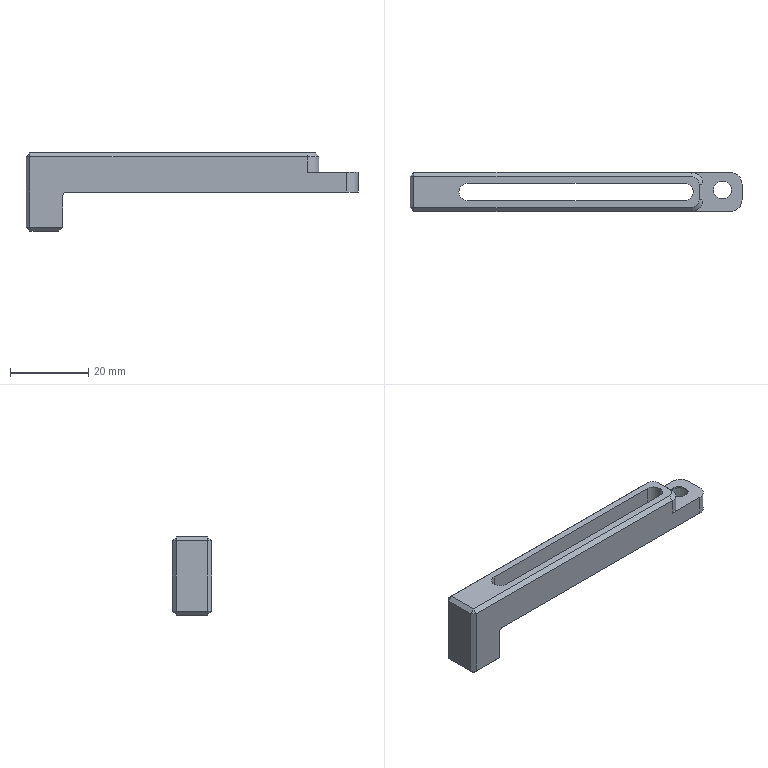Part | SolidWorks | features ICE 4, Fillet 2, HoleWzd 2, Chamfer 1, Extrusion 1 | 1 solid | 51 faces | box 85 x 10 x 20 mm | volume 4776 mm3 | plane 30 | cylinder 17 | cone 4 | commonest cylinder face diameters 4.5 x5 8 x5 6 x4 5 x2 2 x1
STEP:
#1=CARTESIAN_POINT('',(41.5,5.5,-0.4));
#2=VERTEX_POINT('',#1);
#3=CARTESIAN_POINT('',(33.5,5.5,-0.4));
#4=VERTEX_POINT('',#3);
#5=CARTESIAN_POINT('',(37.5,5.5,-0.4));
#6=DIRECTION('',(0.,0.,-1.));
#7=DIRECTION('',(-1.,0.,0.));
#8=AXIS2_PLACEMENT_3D('',#5,#6,#7);
#9=CIRCLE('',#8,4.);
#10=EDGE_CURVE('',#2,#4,#9,.T.);
#11=ORIENTED_EDGE('',*,*,#10,.F.);
#12=CARTESIAN_POINT('',(41.5,5.5,-5.));
#13=VERTEX_POINT('',#12);
#14=CARTESIAN_POINT('',(41.5,5.5,-5.));
#15=DIRECTION('',(0.,0.,-1.));
#16=VECTOR('',#15,1000.);
#17=LINE('',#14,#16);
#18=EDGE_CURVE('',#2,#13,#17,.T.);
#19=ORIENTED_EDGE('',*,*,#18,.T.);
#20=CARTESIAN_POINT('',(33.5,5.5,-5.));
#21=VERTEX_POINT('',#20);
#22=CARTESIAN_POINT('',(37.5,5.5,-5.));
#23=DIRECTION('',(0.,0.,-1.));
#24=DIRECTION('',(-1.,0.,0.));
#25=AXIS2_PLACEMENT_3D('',#22,#23,#24);
#26=CIRCLE('',#25,4.);
#27=EDGE_CURVE('',#13,#21,#26,.T.);
#28=ORIENTED_EDGE('',*,*,#27,.T.);
#29=CARTESIAN_POINT('',(33.5,5.5,-5.));
#30=DIRECTION('',(0.,0.,-1.));
#31=VECTOR('',#30,1000.);
#32=LINE('',#29,#31);
#33=EDGE_CURVE('',#4,#21,#32,.T.);
#34=ORIENTED_EDGE('',*,*,#33,.F.);
#35=EDGE_LOOP('',(#11,#19,#28,#34));
#36=FACE_OUTER_BOUND('',#35,.T.);
#37=CARTESIAN_POINT('',(37.5,5.5,-5.));
#38=DIRECTION('',(0.,0.,-1.));
#39=DIRECTION('',(-1.,0.,0.));
#40=AXIS2_PLACEMENT_3D('',#37,#38,#39);
#41=CYLINDRICAL_SURFACE('',#40,4.);
#42=ADVANCED_FACE('',(#36),#41,.F.);
#43=CARTESIAN_POINT('',(39.75,5.5,0.));
#44=VERTEX_POINT('',#43);
#45=CARTESIAN_POINT('',(35.25,5.5,0.));
#46=VERTEX_POINT('',#45);
#47=CARTESIAN_POINT('',(37.5,5.5,0.));
#48=DIRECTION('',(0.,0.,-1.));
#49=DIRECTION('',(-1.,0.,0.));
#50=AXIS2_PLACEMENT_3D('',#47,#48,#49);
#51=CIRCLE('',#50,2.25);
#52=EDGE_CURVE('',#44,#46,#51,.T.);
#53=ORIENTED_EDGE('',*,*,#52,.F.);
#54=CARTESIAN_POINT('',(39.75,5.5,-0.4));
#55=VERTEX_POINT('',#54);
#56=CARTESIAN_POINT('',(39.75,5.5,-5.));
#57=DIRECTION('',(0.,0.,-1.));
#58=VECTOR('',#57,1000.);
#59=LINE('',#56,#58);
#60=EDGE_CURVE('',#44,#55,#59,.T.);
#61=ORIENTED_EDGE('',*,*,#60,.T.);
#62=CARTESIAN_POINT('',(35.25,5.5,-0.4));
#63=VERTEX_POINT('',#62);
#64=CARTESIAN_POINT('',(37.5,5.5,-0.4));
#65=DIRECTION('',(0.,0.,-1.));
#66=DIRECTION('',(-1.,0.,0.));
#67=AXIS2_PLACEMENT_3D('',#64,#65,#66);
#68=CIRCLE('',#67,2.25);
#69=EDGE_CURVE('',#55,#63,#68,.T.);
#70=ORIENTED_EDGE('',*,*,#69,.T.);
#71=CARTESIAN_POINT('',(35.25,5.5,-5.));
#72=DIRECTION('',(0.,0.,-1.));
#73=VECTOR('',#72,1000.);
#74=LINE('',#71,#73);
#75=EDGE_CURVE('',#46,#63,#74,.T.);
#76=ORIENTED_EDGE('',*,*,#75,.F.);
#77=EDGE_LOOP('',(#53,#61,#70,#76));
#78=FACE_OUTER_BOUND('',#77,.T.);
#79=CARTESIAN_POINT('',(37.5,5.5,-5.));
#80=DIRECTION('',(0.,0.,-1.));
#81=DIRECTION('',(-1.,0.,0.));
#82=AXIS2_PLACEMENT_3D('',#79,#80,#81);
#83=CYLINDRICAL_SURFACE('',#82,2.25);
#84=ADVANCED_FACE('',(#78),#83,.F.);
#85=CARTESIAN_POINT('',(-35.3,4.802,-10.));
#86=VERTEX_POINT('',#85);
#87=CARTESIAN_POINT('',(-40.3,4.802,-10.));
#88=VERTEX_POINT('',#87);
#89=CARTESIAN_POINT('',(-37.8,4.802,-10.));
#90=DIRECTION('',(0.,0.,-1.));
#91=DIRECTION('',(-1.,0.,0.));
#92=AXIS2_PLACEMENT_3D('',#89,#90,#91);
#93=CIRCLE('',#92,2.5);
#94=EDGE_CURVE('',#86,#88,#93,.T.);
#95=ORIENTED_EDGE('',*,*,#94,.F.);
#96=CARTESIAN_POINT('',(-35.3,4.802,-15.));
#97=VERTEX_POINT('',#96);
#98=CARTESIAN_POINT('',(-35.3,4.802,-15.));
#99=DIRECTION('',(0.,0.,-1.));
#100=VECTOR('',#99,1000.);
#101=LINE('',#98,#100);
#102=EDGE_CURVE('',#86,#97,#101,.T.);
#103=ORIENTED_EDGE('',*,*,#102,.T.);
#104=CARTESIAN_POINT('',(-40.3,4.802,-15.));
#105=VERTEX_POINT('',#104);
#106=CARTESIAN_POINT('',(-37.8,4.802,-15.));
#107=DIRECTION('',(0.,0.,-1.));
#108=DIRECTION('',(-1.,0.,0.));
#109=AXIS2_PLACEMENT_3D('',#106,#107,#108);
#110=CIRCLE('',#109,2.5);
#111=EDGE_CURVE('',#97,#105,#110,.T.);
#112=ORIENTED_EDGE('',*,*,#111,.T.);
#113=CARTESIAN_POINT('',(-40.3,4.802,-15.));
#114=DIRECTION('',(0.,0.,-1.));
#115=VECTOR('',#114,1000.);
#116=LINE('',#113,#115);
#117=EDGE_CURVE('',#88,#105,#116,.T.);
#118=ORIENTED_EDGE('',*,*,#117,.F.);
#119=EDGE_LOOP('',(#95,#103,#112,#118));
#120=FACE_OUTER_BOUND('',#119,.T.);
#121=CARTESIAN_POINT('',(-37.8,4.802,-15.));
#122=DIRECTION('',(0.,0.,-1.));
#123=DIRECTION('',(-1.,0.,0.));
#124=AXIS2_PLACEMENT_3D('',#121,#122,#123);
#125=CYLINDRICAL_SURFACE('',#124,2.5);
#126=ADVANCED_FACE('',(#120),#125,.F.);
#127=CARTESIAN_POINT('',(-37.8,4.802,-8.498));
#128=VERTEX_POINT('',#127);
#129=CARTESIAN_POINT('',(-40.3,4.802,-10.));
#130=DIRECTION('',(-0.8572,0.,-0.515));
#131=VECTOR('',#130,1000.);
#132=LINE('',#129,#131);
#133=EDGE_CURVE('',#128,#88,#132,.T.);
#134=ORIENTED_EDGE('',*,*,#133,.F.);
#135=CARTESIAN_POINT('',(-35.3,4.802,-10.));
#136=DIRECTION('',(0.8572,0.,-0.515));
#137=VECTOR('',#136,1000.);
#138=LINE('',#135,#137);
#139=EDGE_CURVE('',#128,#86,#138,.T.);
#140=ORIENTED_EDGE('',*,*,#139,.T.);
#141=ORIENTED_EDGE('',*,*,#94,.T.);
#142=EDGE_LOOP('',(#134,#140,#141));
#143=FACE_OUTER_BOUND('',#142,.T.);
#144=CARTESIAN_POINT('',(-37.8,4.802,-10.));
#145=DIRECTION('',(0.,0.,-1.));
#146=DIRECTION('',(-1.,0.,0.));
#147=AXIS2_PLACEMENT_3D('',#144,#145,#146);
#148=CONICAL_SURFACE('',#147,2.5,1.03);
#149=ADVANCED_FACE('',(#143),#148,.F.);
#150=CARTESIAN_POINT('',(-30.,5.,5.));
#151=VERTEX_POINT('',#150);
#152=CARTESIAN_POINT('',(-27.75,7.25,5.));
#153=VERTEX_POINT('',#152);
#154=CARTESIAN_POINT('',(-27.75,5.,5.));
#155=DIRECTION('',(0.,0.,-1.));
#156=DIRECTION('',(-1.,0.,0.));
#157=AXIS2_PLACEMENT_3D('',#154,#155,#156);
#158=CIRCLE('',#157,2.25);
#159=EDGE_CURVE('',#151,#153,#158,.T.);
#160=ORIENTED_EDGE('',*,*,#159,.F.);
#161=CARTESIAN_POINT('',(-30.,5.,-0.6));
#162=VERTEX_POINT('',#161);
#163=CARTESIAN_POINT('',(-30.,5.,5.));
#164=DIRECTION('',(0.,0.,-1.));
#165=VECTOR('',#164,1000.);
#166=LINE('',#163,#165);
#167=EDGE_CURVE('',#151,#162,#166,.T.);
#168=ORIENTED_EDGE('',*,*,#167,.T.);
#169=CARTESIAN_POINT('',(-27.75,7.25,-0.6));
#170=VERTEX_POINT('',#169);
#171=CARTESIAN_POINT('',(-27.75,5.,-0.6));
#172=DIRECTION('',(0.,0.,-1.));
#173=DIRECTION('',(-1.,0.,0.));
#174=AXIS2_PLACEMENT_3D('',#171,#172,#173);
#175=CIRCLE('',#174,2.25);
#176=EDGE_CURVE('',#162,#170,#175,.T.);
#177=ORIENTED_EDGE('',*,*,#176,.T.);
#178=CARTESIAN_POINT('',(-27.75,7.25,5.));
#179=DIRECTION('',(0.,0.,-1.));
#180=VECTOR('',#179,1000.);
#181=LINE('',#178,#180);
#182=EDGE_CURVE('',#153,#170,#181,.T.);
#183=ORIENTED_EDGE('',*,*,#182,.F.);
#184=EDGE_LOOP('',(#160,#168,#177,#183));
#185=FACE_OUTER_BOUND('',#184,.T.);
#186=CARTESIAN_POINT('',(-27.75,5.,5.));
#187=DIRECTION('',(0.,0.,-1.));
#188=DIRECTION('',(-1.,0.,0.));
#189=AXIS2_PLACEMENT_3D('',#186,#187,#188);
#190=CYLINDRICAL_SURFACE('',#189,2.25);
#191=ADVANCED_FACE('',(#185),#190,.F.);
#192=CARTESIAN_POINT('',(-27.75,9.,-0.6));
#193=VERTEX_POINT('',#192);
#194=CARTESIAN_POINT('',(-31.75,5.,-0.6));
#195=VERTEX_POINT('',#194);
#196=CARTESIAN_POINT('',(-27.75,5.,-0.6));
#197=DIRECTION('',(0.,0.,1.));
#198=DIRECTION('',(1.,0.,0.));
#199=AXIS2_PLACEMENT_3D('',#196,#197,#198);
#200=CIRCLE('',#199,4.);
#201=EDGE_CURVE('',#193,#195,#200,.T.);
#202=ORIENTED_EDGE('',*,*,#201,.T.);
#203=CARTESIAN_POINT('',(-31.75,5.,-5.));
#204=VERTEX_POINT('',#203);
#205=CARTESIAN_POINT('',(-31.75,5.,-0.6));
#206=DIRECTION('',(0.,0.,-1.));
#207=VECTOR('',#206,1000.);
#208=LINE('',#205,#207);
#209=EDGE_CURVE('',#195,#204,#208,.T.);
#210=ORIENTED_EDGE('',*,*,#209,.T.);
#211=CARTESIAN_POINT('',(-27.75,9.,-5.));
#212=VERTEX_POINT('',#211);
#213=CARTESIAN_POINT('',(-27.75,5.,-5.));
#214=DIRECTION('',(0.,0.,1.));
#215=DIRECTION('',(1.,0.,0.));
#216=AXIS2_PLACEMENT_3D('',#213,#214,#215);
#217=CIRCLE('',#216,4.);
#218=EDGE_CURVE('',#212,#204,#217,.T.);
#219=ORIENTED_EDGE('',*,*,#218,.F.);
#220=CARTESIAN_POINT('',(-27.75,9.,-0.6));
#221=DIRECTION('',(0.,0.,-1.));
#222=VECTOR('',#221,1000.);
#223=LINE('',#220,#222);
#224=EDGE_CURVE('',#193,#212,#223,.T.);
#225=ORIENTED_EDGE('',*,*,#224,.F.);
#226=EDGE_LOOP('',(#202,#210,#219,#225));
#227=FACE_OUTER_BOUND('',#226,.T.);
#228=CARTESIAN_POINT('',(-27.75,5.,-0.6));
#229=DIRECTION('',(0.,0.,-1.));
#230=DIRECTION('',(-1.,0.,0.));
#231=AXIS2_PLACEMENT_3D('',#228,#229,#230);
#232=CYLINDRICAL_SURFACE('',#231,4.);
#233=ADVANCED_FACE('',(#227),#232,.F.);
#234=CARTESIAN_POINT('',(37.5,5.5,-5.));
#235=DIRECTION('',(0.,0.,-1.));
#236=DIRECTION('',(-1.,0.,0.));
#237=AXIS2_PLACEMENT_3D('',#234,#235,#236);
#238=CIRCLE('',#237,4.);
#239=EDGE_CURVE('',#21,#13,#238,.T.);
#240=ORIENTED_EDGE('',*,*,#239,.F.);
#241=ORIENTED_EDGE('',*,*,#27,.F.);
#242=EDGE_LOOP('',(#240,#241));
#243=FACE_BOUND('',#242,.T.);
#244=ORIENTED_EDGE('',*,*,#218,.T.);
#245=CARTESIAN_POINT('',(-27.75,1.,-5.));
#246=VERTEX_POINT('',#245);
#247=CARTESIAN_POINT('',(-27.75,5.,-5.));
#248=DIRECTION('',(0.,0.,1.));
#249=DIRECTION('',(1.,0.,0.));
#250=AXIS2_PLACEMENT_3D('',#247,#248,#249);
#251=CIRCLE('',#250,4.);
#252=EDGE_CURVE('',#204,#246,#251,.T.);
#253=ORIENTED_EDGE('',*,*,#252,.T.);
#254=CARTESIAN_POINT('',(27.75,1.,-5.));
#255=VERTEX_POINT('',#254);
#256=CARTESIAN_POINT('',(-27.75,1.,-5.));
#257=DIRECTION('',(1.,0.,0.));
#258=VECTOR('',#257,1000.);
#259=LINE('',#256,#258);
#260=EDGE_CURVE('',#246,#255,#259,.T.);
#261=ORIENTED_EDGE('',*,*,#260,.T.);
#262=CARTESIAN_POINT('',(27.75,9.,-5.));
#263=VERTEX_POINT('',#262);
#264=CARTESIAN_POINT('',(27.75,5.,-5.));
#265=DIRECTION('',(0.,0.,1.));
#266=DIRECTION('',(1.,0.,0.));
#267=AXIS2_PLACEMENT_3D('',#264,#265,#266);
#268=CIRCLE('',#267,4.);
#269=EDGE_CURVE('',#255,#263,#268,.T.);
#270=ORIENTED_EDGE('',*,*,#269,.T.);
#271=CARTESIAN_POINT('',(-27.75,9.,-5.));
#272=DIRECTION('',(-1.,0.,0.));
#273=VECTOR('',#272,1000.);
#274=LINE('',#271,#273);
#275=EDGE_CURVE('',#263,#212,#274,.T.);
#276=ORIENTED_EDGE('',*,*,#275,.T.);
#277=EDGE_LOOP('',(#244,#253,#261,#270,#276));
#278=FACE_BOUND('',#277,.T.);
#279=CARTESIAN_POINT('',(39.5,0.,-5.));
#280=VERTEX_POINT('',#279);
#281=CARTESIAN_POINT('',(-32.1,0.,-5.));
#282=VERTEX_POINT('',#281);
#283=CARTESIAN_POINT('',(42.5,0.,-5.));
#284=DIRECTION('',(-1.,0.,0.));
#285=VECTOR('',#284,1000.);
#286=LINE('',#283,#285);
#287=EDGE_CURVE('',#280,#282,#286,.T.);
#288=ORIENTED_EDGE('',*,*,#287,.T.);
#289=CARTESIAN_POINT('',(-32.1,10.,-5.));
#290=VERTEX_POINT('',#289);
#291=CARTESIAN_POINT('',(-32.1,10.,-5.));
#292=DIRECTION('',(0.,1.,0.));
#293=VECTOR('',#292,1000.);
#294=LINE('',#291,#293);
#295=EDGE_CURVE('',#282,#290,#294,.T.);
#296=ORIENTED_EDGE('',*,*,#295,.T.);
#297=CARTESIAN_POINT('',(39.5,10.,-5.));
#298=VERTEX_POINT('',#297);
#299=CARTESIAN_POINT('',(42.5,10.,-5.));
#300=DIRECTION('',(-1.,0.,0.));
#301=VECTOR('',#300,1000.);
#302=LINE('',#299,#301);
#303=EDGE_CURVE('',#298,#290,#302,.T.);
#304=ORIENTED_EDGE('',*,*,#303,.F.);
#305=CARTESIAN_POINT('',(42.5,7.,-5.));
#306=VERTEX_POINT('',#305);
#307=CARTESIAN_POINT('',(39.5,7.,-5.));
#308=DIRECTION('',(0.,0.,-1.));
#309=DIRECTION('',(1.,0.,0.));
#310=AXIS2_PLACEMENT_3D('',#307,#308,#309);
#311=CIRCLE('',#310,3.);
#312=EDGE_CURVE('',#298,#306,#311,.T.);
#313=ORIENTED_EDGE('',*,*,#312,.T.);
#314=CARTESIAN_POINT('',(42.5,3.,-5.));
#315=VERTEX_POINT('',#314);
#316=CARTESIAN_POINT('',(42.5,10.,-5.));
#317=DIRECTION('',(0.,-1.,0.));
#318=VECTOR('',#317,1000.);
#319=LINE('',#316,#318);
#320=EDGE_CURVE('',#306,#315,#319,.T.);
#321=ORIENTED_EDGE('',*,*,#320,.T.);
#322=CARTESIAN_POINT('',(39.5,3.,-5.));
#323=DIRECTION('',(0.,0.,-1.));
#324=DIRECTION('',(1.,0.,0.));
#325=AXIS2_PLACEMENT_3D('',#322,#323,#324);
#326=CIRCLE('',#325,3.);
#327=EDGE_CURVE('',#315,#280,#326,.T.);
#328=ORIENTED_EDGE('',*,*,#327,.T.);
#329=EDGE_LOOP('',(#288,#296,#304,#313,#321,#328));
#330=FACE_OUTER_BOUND('',#329,.T.);
#331=CARTESIAN_POINT('',(42.5,10.,-5.));
#332=DIRECTION('',(0.,0.,1.));
#333=DIRECTION('',(1.,0.,0.));
#334=AXIS2_PLACEMENT_3D('',#331,#332,#333);
#335=PLANE('',#334);
#336=ADVANCED_FACE('',(#243,#278,#330),#335,.F.);
#337=ORIENTED_EDGE('',*,*,#201,.F.);
#338=CARTESIAN_POINT('',(27.75,9.,-0.6));
#339=VERTEX_POINT('',#338);
#340=CARTESIAN_POINT('',(-27.75,9.,-0.6));
#341=DIRECTION('',(-1.,0.,0.));
#342=VECTOR('',#341,1000.);
#343=LINE('',#340,#342);
#344=EDGE_CURVE('',#339,#193,#343,.T.);
#345=ORIENTED_EDGE('',*,*,#344,.F.);
#346=CARTESIAN_POINT('',(27.75,1.,-0.6));
#347=VERTEX_POINT('',#346);
#348=CARTESIAN_POINT('',(27.75,5.,-0.6));
#349=DIRECTION('',(0.,0.,1.));
#350=DIRECTION('',(1.,0.,0.));
#351=AXIS2_PLACEMENT_3D('',#348,#349,#350);
#352=CIRCLE('',#351,4.);
#353=EDGE_CURVE('',#347,#339,#352,.T.);
#354=ORIENTED_EDGE('',*,*,#353,.F.);
#355=CARTESIAN_POINT('',(-27.75,1.,-0.6));
#356=VERTEX_POINT('',#355);
#357=CARTESIAN_POINT('',(-27.75,1.,-0.6));
#358=DIRECTION('',(1.,0.,0.));
#359=VECTOR('',#358,1000.);
#360=LINE('',#357,#359);
#361=EDGE_CURVE('',#356,#347,#360,.T.);
#362=ORIENTED_EDGE('',*,*,#361,.F.);
#363=CARTESIAN_POINT('',(-27.75,5.,-0.6));
#364=DIRECTION('',(0.,0.,1.));
#365=DIRECTION('',(1.,0.,0.));
#366=AXIS2_PLACEMENT_3D('',#363,#364,#365);
#367=CIRCLE('',#366,4.);
#368=EDGE_CURVE('',#195,#356,#367,.T.);
#369=ORIENTED_EDGE('',*,*,#368,.F.);
#370=EDGE_LOOP('',(#337,#345,#354,#362,#369));
#371=FACE_OUTER_BOUND('',#370,.T.);
#372=CARTESIAN_POINT('',(27.75,7.25,-0.6));
#373=VERTEX_POINT('',#372);
#374=CARTESIAN_POINT('',(27.75,2.75,-0.6));
#375=VERTEX_POINT('',#374);
#376=CARTESIAN_POINT('',(27.75,5.,-0.6));
#377=DIRECTION('',(0.,0.,-1.));
#378=DIRECTION('',(-1.,0.,0.));
#379=AXIS2_PLACEMENT_3D('',#376,#377,#378);
#380=CIRCLE('',#379,2.25);
#381=EDGE_CURVE('',#373,#375,#380,.T.);
#382=ORIENTED_EDGE('',*,*,#381,.F.);
#383=CARTESIAN_POINT('',(27.75,7.25,-0.6));
#384=DIRECTION('',(1.,0.,0.));
#385=VECTOR('',#384,1000.);
#386=LINE('',#383,#385);
#387=EDGE_CURVE('',#170,#373,#386,.T.);
#388=ORIENTED_EDGE('',*,*,#387,.F.);
#389=ORIENTED_EDGE('',*,*,#176,.F.);
#390=CARTESIAN_POINT('',(-27.75,2.75,-0.6));
#391=VERTEX_POINT('',#390);
#392=CARTESIAN_POINT('',(-27.75,5.,-0.6));
#393=DIRECTION('',(0.,0.,-1.));
#394=DIRECTION('',(-1.,0.,0.));
#395=AXIS2_PLACEMENT_3D('',#392,#393,#394);
#396=CIRCLE('',#395,2.25);
#397=EDGE_CURVE('',#391,#162,#396,.T.);
#398=ORIENTED_EDGE('',*,*,#397,.F.);
#399=CARTESIAN_POINT('',(27.75,2.75,-0.6));
#400=DIRECTION('',(-1.,0.,0.));
#401=VECTOR('',#400,1000.);
#402=LINE('',#399,#401);
#403=EDGE_CURVE('',#375,#391,#402,.T.);
#404=ORIENTED_EDGE('',*,*,#403,.F.);
#405=EDGE_LOOP('',(#382,#388,#389,#398,#404));
#406=FACE_BOUND('',#405,.T.);
#407=CARTESIAN_POINT('',(-27.75,5.,-0.6));
#408=DIRECTION('',(0.,0.,1.));
#409=DIRECTION('',(1.,0.,0.));
#410=AXIS2_PLACEMENT_3D('',#407,#408,#409);
#411=PLANE('',#410);
#412=ADVANCED_FACE('',(#371,#406),#411,.F.);
#413=CARTESIAN_POINT('',(-42.5,9.,-14.));
#414=VERTEX_POINT('',#413);
#415=CARTESIAN_POINT('',(-42.5,1.,-14.));
#416=VERTEX_POINT('',#415);
#417=CARTESIAN_POINT('',(-42.5,0.,-14.));
#418=DIRECTION('',(0.,-1.,0.));
#419=VECTOR('',#418,1000.);
#420=LINE('',#417,#419);
#421=EDGE_CURVE('',#414,#416,#420,.T.);
#422=ORIENTED_EDGE('',*,*,#421,.T.);
#423=CARTESIAN_POINT('',(-42.5,1.,4.));
#424=VERTEX_POINT('',#423);
#425=CARTESIAN_POINT('',(-42.5,1.,5.));
#426=DIRECTION('',(0.,0.,1.));
#427=VECTOR('',#426,1000.);
#428=LINE('',#425,#427);
#429=EDGE_CURVE('',#416,#424,#428,.T.);
#430=ORIENTED_EDGE('',*,*,#429,.T.);
#431=CARTESIAN_POINT('',(-42.5,9.,4.));
#432=VERTEX_POINT('',#431);
#433=CARTESIAN_POINT('',(-42.5,10.,4.));
#434=DIRECTION('',(0.,1.,0.));
#435=VECTOR('',#434,1000.);
#436=LINE('',#433,#435);
#437=EDGE_CURVE('',#424,#432,#436,.T.);
#438=ORIENTED_EDGE('',*,*,#437,.T.);
#439=CARTESIAN_POINT('',(-42.5,9.,-15.));
#440=DIRECTION('',(0.,0.,-1.));
#441=VECTOR('',#440,1000.);
#442=LINE('',#439,#441);
#443=EDGE_CURVE('',#432,#414,#442,.T.);
#444=ORIENTED_EDGE('',*,*,#443,.T.);
#445=EDGE_LOOP('',(#422,#430,#438,#444));
#446=FACE_OUTER_BOUND('',#445,.T.);
#447=CARTESIAN_POINT('',(-42.5,10.,5.));
#448=DIRECTION('',(1.,0.,0.));
#449=DIRECTION('',(0.,0.,-1.));
#450=AXIS2_PLACEMENT_3D('',#447,#448,#449);
#451=PLANE('',#450);
#452=ADVANCED_FACE('',(#446),#451,.F.);
#453=CARTESIAN_POINT('',(29.5,1.,5.));
#454=VERTEX_POINT('',#453);
#455=CARTESIAN_POINT('',(31.5,3.,5.));
#456=VERTEX_POINT('',#455);
#457=CARTESIAN_POINT('',(29.5,3.,5.));
#458=DIRECTION('',(0.,0.,1.));
#459=DIRECTION('',(-1.,0.,0.));
#460=AXIS2_PLACEMENT_3D('',#457,#458,#459);
#461=CIRCLE('',#460,2.);
#462=EDGE_CURVE('',#454,#456,#461,.T.);
#463=ORIENTED_EDGE('',*,*,#462,.T.);
#464=CARTESIAN_POINT('',(31.5,7.,5.));
#465=VERTEX_POINT('',#464);
#466=CARTESIAN_POINT('',(31.5,10.,5.));
#467=DIRECTION('',(0.,1.,0.));
#468=VECTOR('',#467,1000.);
#469=LINE('',#466,#468);
#470=EDGE_CURVE('',#456,#465,#469,.T.);
#471=ORIENTED_EDGE('',*,*,#470,.T.);
#472=CARTESIAN_POINT('',(29.5,9.,5.));
#473=VERTEX_POINT('',#472);
#474=CARTESIAN_POINT('',(29.5,7.,5.));
#475=DIRECTION('',(0.,0.,1.));
#476=DIRECTION('',(-1.,0.,0.));
#477=AXIS2_PLACEMENT_3D('',#474,#475,#476);
#478=CIRCLE('',#477,2.);
#479=EDGE_CURVE('',#465,#473,#478,.T.);
#480=ORIENTED_EDGE('',*,*,#479,.T.);
#481=CARTESIAN_POINT('',(-41.5,9.,5.));
#482=VERTEX_POINT('',#481);
#483=CARTESIAN_POINT('',(-42.5,9.,5.));
#484=DIRECTION('',(-1.,0.,0.));
#485=VECTOR('',#484,1000.);
#486=LINE('',#483,#485);
#487=EDGE_CURVE('',#473,#482,#486,.T.);
#488=ORIENTED_EDGE('',*,*,#487,.T.);
#489=CARTESIAN_POINT('',(-41.5,1.,5.));
#490=VERTEX_POINT('',#489);
#491=CARTESIAN_POINT('',(-41.5,10.,5.));
#492=DIRECTION('',(0.,-1.,0.));
#493=VECTOR('',#492,1000.);
#494=LINE('',#491,#493);
#495=EDGE_CURVE('',#482,#490,#494,.T.);
#496=ORIENTED_EDGE('',*,*,#495,.T.);
#497=CARTESIAN_POINT('',(42.5,1.,5.));
#498=DIRECTION('',(1.,0.,0.));
#499=VECTOR('',#498,1000.);
#500=LINE('',#497,#499);
#501=EDGE_CURVE('',#490,#454,#500,.T.);
#502=ORIENTED_EDGE('',*,*,#501,.T.);
#503=EDGE_LOOP('',(#463,#471,#480,#488,#496,#502));
#504=FACE_OUTER_BOUND('',#503,.T.);
#505=CARTESIAN_POINT('',(27.75,7.25,5.));
#506=VERTEX_POINT('',#505);
#507=CARTESIAN_POINT('',(27.75,7.25,5.));
#508=DIRECTION('',(1.,0.,0.));
#509=VECTOR('',#508,1000.);
#510=LINE('',#507,#509);
#511=EDGE_CURVE('',#153,#506,#510,.T.);
#512=ORIENTED_EDGE('',*,*,#511,.T.);
#513=CARTESIAN_POINT('',(27.75,2.75,5.));
#514=VERTEX_POINT('',#513);
#515=CARTESIAN_POINT('',(27.75,5.,5.));
#516=DIRECTION('',(0.,0.,-1.));
#517=DIRECTION('',(-1.,0.,0.));
#518=AXIS2_PLACEMENT_3D('',#515,#516,#517);
#519=CIRCLE('',#518,2.25);
#520=EDGE_CURVE('',#506,#514,#519,.T.);
#521=ORIENTED_EDGE('',*,*,#520,.T.);
#522=CARTESIAN_POINT('',(-27.75,2.75,5.));
#523=VERTEX_POINT('',#522);
#524=CARTESIAN_POINT('',(27.75,2.75,5.));
#525=DIRECTION('',(-1.,0.,0.));
#526=VECTOR('',#525,1000.);
#527=LINE('',#524,#526);
#528=EDGE_CURVE('',#514,#523,#527,.T.);
#529=ORIENTED_EDGE('',*,*,#528,.T.);
#530=CARTESIAN_POINT('',(-27.75,5.,5.));
#531=DIRECTION('',(0.,0.,-1.));
#532=DIRECTION('',(-1.,0.,0.));
#533=AXIS2_PLACEMENT_3D('',#530,#531,#532);
#534=CIRCLE('',#533,2.25);
#535=EDGE_CURVE('',#523,#151,#534,.T.);
#536=ORIENTED_EDGE('',*,*,#535,.T.);
#537=ORIENTED_EDGE('',*,*,#159,.T.);
#538=EDGE_LOOP('',(#512,#521,#529,#536,#537));
#539=FACE_BOUND('',#538,.T.);
#540=CARTESIAN_POINT('',(42.5,10.,5.));
#541=DIRECTION('',(0.,0.,-1.));
#542=DIRECTION('',(-1.,0.,0.));
#543=AXIS2_PLACEMENT_3D('',#540,#541,#542);
#544=PLANE('',#543);
#545=ADVANCED_FACE('',(#504,#539),#544,.F.);
#546=CARTESIAN_POINT('',(42.5,3.,0.));
#547=VERTEX_POINT('',#546);
#548=CARTESIAN_POINT('',(42.5,7.,0.));
#549=VERTEX_POINT('',#548);
#550=CARTESIAN_POINT('',(42.5,10.,0.));
#551=DIRECTION('',(0.,1.,0.));
#552=VECTOR('',#551,1000.);
#553=LINE('',#550,#552);
#554=EDGE_CURVE('',#547,#549,#553,.T.);
#555=ORIENTED_EDGE('',*,*,#554,.F.);
#556=CARTESIAN_POINT('',(42.5,3.,5.));
#557=DIRECTION('',(0.,0.,-1.));
#558=VECTOR('',#557,1000.);
#559=LINE('',#556,#558);
#560=EDGE_CURVE('',#547,#315,#559,.T.);
#561=ORIENTED_EDGE('',*,*,#560,.T.);
#562=ORIENTED_EDGE('',*,*,#320,.F.);
#563=CARTESIAN_POINT('',(42.5,7.,0.));
#564=DIRECTION('',(0.,0.,1.));
#565=VECTOR('',#564,1000.);
#566=LINE('',#563,#565);
#567=EDGE_CURVE('',#306,#549,#566,.T.);
#568=ORIENTED_EDGE('',*,*,#567,.T.);
#569=EDGE_LOOP('',(#555,#561,#562,#568));
#570=FACE_OUTER_BOUND('',#569,.T.);
#571=CARTESIAN_POINT('',(42.5,10.,5.));
#572=DIRECTION('',(-1.,0.,0.));
#573=DIRECTION('',(0.,0.,1.));
#574=AXIS2_PLACEMENT_3D('',#571,#572,#573);
#575=PLANE('',#574);
#576=ADVANCED_FACE('',(#570),#575,.F.);
#577=CARTESIAN_POINT('',(-41.5,10.,-14.));
#578=VERTEX_POINT('',#577);
#579=CARTESIAN_POINT('',(-41.5,10.,4.));
#580=VERTEX_POINT('',#579);
#581=CARTESIAN_POINT('',(-41.5,10.,5.));
#582=DIRECTION('',(0.,0.,1.));
#583=VECTOR('',#582,1000.);
#584=LINE('',#581,#583);
#585=EDGE_CURVE('',#578,#580,#584,.T.);
#586=ORIENTED_EDGE('',*,*,#585,.T.);
#587=CARTESIAN_POINT('',(29.5,10.,4.));
#588=VERTEX_POINT('',#587);
#589=CARTESIAN_POINT('',(29.5,10.,4.));
#590=DIRECTION('',(1.,0.,0.));
#591=VECTOR('',#590,1000.);
#592=LINE('',#589,#591);
#593=EDGE_CURVE('',#580,#588,#592,.T.);
#594=ORIENTED_EDGE('',*,*,#593,.T.);
#595=CARTESIAN_POINT('',(29.5,10.,0.));
#596=VERTEX_POINT('',#595);
#597=CARTESIAN_POINT('',(29.5,10.,0.));
#598=DIRECTION('',(0.,0.,-1.));
#599=VECTOR('',#598,1000.);
#600=LINE('',#597,#599);
#601=EDGE_CURVE('',#588,#596,#600,.T.);
#602=ORIENTED_EDGE('',*,*,#601,.T.);
#603=CARTESIAN_POINT('',(39.5,10.,0.));
#604=VERTEX_POINT('',#603);
#605=CARTESIAN_POINT('',(42.5,10.,0.));
#606=DIRECTION('',(-1.,0.,0.));
#607=VECTOR('',#606,1000.);
#608=LINE('',#605,#607);
#609=EDGE_CURVE('',#604,#596,#608,.T.);
#610=ORIENTED_EDGE('',*,*,#609,.F.);
#611=CARTESIAN_POINT('',(39.5,10.,-5.));
#612=DIRECTION('',(0.,0.,-1.));
#613=VECTOR('',#612,1000.);
#614=LINE('',#611,#613);
#615=EDGE_CURVE('',#604,#298,#614,.T.);
#616=ORIENTED_EDGE('',*,*,#615,.T.);
#617=ORIENTED_EDGE('',*,*,#303,.T.);
#618=CARTESIAN_POINT('',(-33.1,10.,-6.));
#619=VERTEX_POINT('',#618);
#620=CARTESIAN_POINT('',(-32.1,10.,-6.));
#621=DIRECTION('',(0.,-1.,0.));
#622=DIRECTION('',(0.,0.,1.));
#623=AXIS2_PLACEMENT_3D('',#620,#621,#622);
#624=CIRCLE('',#623,1.);
#625=EDGE_CURVE('',#290,#619,#624,.T.);
#626=ORIENTED_EDGE('',*,*,#625,.T.);
#627=CARTESIAN_POINT('',(-33.1,10.,-14.));
#628=VERTEX_POINT('',#627);
#629=CARTESIAN_POINT('',(-33.1,10.,-15.));
#630=DIRECTION('',(0.,0.,1.));
#631=VECTOR('',#630,1000.);
#632=LINE('',#629,#631);
#633=EDGE_CURVE('',#628,#619,#632,.T.);
#634=ORIENTED_EDGE('',*,*,#633,.F.);
#635=CARTESIAN_POINT('',(0.,10.,-14.));
#636=DIRECTION('',(-1.,0.,0.));
#637=VECTOR('',#636,1000.);
#638=LINE('',#635,#637);
#639=EDGE_CURVE('',#628,#578,#638,.T.);
#640=ORIENTED_EDGE('',*,*,#639,.T.);
#641=EDGE_LOOP('',(#586,#594,#602,#610,#616,#617,#626,#634,#640));
#642=FACE_OUTER_BOUND('',#641,.T.);
#643=CARTESIAN_POINT('',(0.,10.,0.));
#644=DIRECTION('',(0.,1.,0.));
#645=DIRECTION('',(0.,0.,1.));
#646=AXIS2_PLACEMENT_3D('',#643,#644,#645);
#647=PLANE('',#646);
#648=ADVANCED_FACE('',(#642),#647,.T.);
#649=CARTESIAN_POINT('',(29.5,0.,0.));
#650=VERTEX_POINT('',#649);
#651=CARTESIAN_POINT('',(29.5,0.,4.));
#652=VERTEX_POINT('',#651);
#653=CARTESIAN_POINT('',(29.5,0.,0.));
#654=DIRECTION('',(0.,0.,1.));
#655=VECTOR('',#654,1000.);
#656=LINE('',#653,#655);
#657=EDGE_CURVE('',#650,#652,#656,.T.);
#658=ORIENTED_EDGE('',*,*,#657,.T.);
#659=CARTESIAN_POINT('',(-41.5,0.,4.));
#660=VERTEX_POINT('',#659);
#661=CARTESIAN_POINT('',(0.,0.,4.));
#662=DIRECTION('',(-1.,0.,0.));
#663=VECTOR('',#662,1000.);
#664=LINE('',#661,#663);
#665=EDGE_CURVE('',#652,#660,#664,.T.);
#666=ORIENTED_EDGE('',*,*,#665,.T.);
#667=CARTESIAN_POINT('',(-41.5,0.,-14.));
#668=VERTEX_POINT('',#667);
#669=CARTESIAN_POINT('',(-41.5,0.,0.));
#670=DIRECTION('',(0.,0.,-1.));
#671=VECTOR('',#670,1000.);
#672=LINE('',#669,#671);
#673=EDGE_CURVE('',#660,#668,#672,.T.);
#674=ORIENTED_EDGE('',*,*,#673,.T.);
#675=CARTESIAN_POINT('',(-33.1,0.,-14.));
#676=VERTEX_POINT('',#675);
#677=CARTESIAN_POINT('',(-33.1,0.,-14.));
#678=DIRECTION('',(1.,0.,0.));
#679=VECTOR('',#678,1000.);
#680=LINE('',#677,#679);
#681=EDGE_CURVE('',#668,#676,#680,.T.);
#682=ORIENTED_EDGE('',*,*,#681,.T.);
#683=CARTESIAN_POINT('',(-33.1,0.,-6.));
#684=VERTEX_POINT('',#683);
#685=CARTESIAN_POINT('',(-33.1,0.,-15.));
#686=DIRECTION('',(0.,0.,1.));
#687=VECTOR('',#686,1000.);
#688=LINE('',#685,#687);
#689=EDGE_CURVE('',#676,#684,#688,.T.);
#690=ORIENTED_EDGE('',*,*,#689,.T.);
#691=CARTESIAN_POINT('',(-32.1,0.,-6.));
#692=DIRECTION('',(0.,1.,0.));
#693=DIRECTION('',(0.,0.,1.));
#694=AXIS2_PLACEMENT_3D('',#691,#692,#693);
#695=CIRCLE('',#694,1.);
#696=EDGE_CURVE('',#684,#282,#695,.T.);
#697=ORIENTED_EDGE('',*,*,#696,.T.);
#698=ORIENTED_EDGE('',*,*,#287,.F.);
#699=CARTESIAN_POINT('',(39.5,0.,0.));
#700=VERTEX_POINT('',#699);
#701=CARTESIAN_POINT('',(39.5,0.,0.));
#702=DIRECTION('',(0.,0.,1.));
#703=VECTOR('',#702,1000.);
#704=LINE('',#701,#703);
#705=EDGE_CURVE('',#280,#700,#704,.T.);
#706=ORIENTED_EDGE('',*,*,#705,.T.);
#707=CARTESIAN_POINT('',(42.5,0.,0.));
#708=DIRECTION('',(1.,0.,0.));
#709=VECTOR('',#708,1000.);
#710=LINE('',#707,#709);
#711=EDGE_CURVE('',#650,#700,#710,.T.);
#712=ORIENTED_EDGE('',*,*,#711,.F.);
#713=EDGE_LOOP('',(#658,#666,#674,#682,#690,#697,#698,#706,#712));
#714=FACE_OUTER_BOUND('',#713,.T.);
#715=CARTESIAN_POINT('',(0.,0.,0.));
#716=DIRECTION('',(0.,1.,0.));
#717=DIRECTION('',(0.,0.,1.));
#718=AXIS2_PLACEMENT_3D('',#715,#716,#717);
#719=PLANE('',#718);
#720=ADVANCED_FACE('',(#714),#719,.F.);
#721=ORIENTED_EDGE('',*,*,#209,.F.);
#722=ORIENTED_EDGE('',*,*,#368,.T.);
#723=CARTESIAN_POINT('',(-27.75,1.,-0.6));
#724=DIRECTION('',(0.,0.,-1.));
#725=VECTOR('',#724,1000.);
#726=LINE('',#723,#725);
#727=EDGE_CURVE('',#356,#246,#726,.T.);
#728=ORIENTED_EDGE('',*,*,#727,.T.);
#729=ORIENTED_EDGE('',*,*,#252,.F.);
#730=EDGE_LOOP('',(#721,#722,#728,#729));
#731=FACE_OUTER_BOUND('',#730,.T.);
#732=CARTESIAN_POINT('',(-27.75,5.,-0.6));
#733=DIRECTION('',(0.,0.,-1.));
#734=DIRECTION('',(-1.,0.,0.));
#735=AXIS2_PLACEMENT_3D('',#732,#733,#734);
#736=CYLINDRICAL_SURFACE('',#735,4.);
#737=ADVANCED_FACE('',(#731),#736,.F.);
#738=ORIENTED_EDGE('',*,*,#260,.F.);
#739=ORIENTED_EDGE('',*,*,#727,.F.);
#740=ORIENTED_EDGE('',*,*,#361,.T.);
#741=CARTESIAN_POINT('',(27.75,1.,-0.6));
#742=DIRECTION('',(0.,0.,-1.));
#743=VECTOR('',#742,1000.);
#744=LINE('',#741,#743);
#745=EDGE_CURVE('',#347,#255,#744,.T.);
#746=ORIENTED_EDGE('',*,*,#745,.T.);
#747=EDGE_LOOP('',(#738,#739,#740,#746));
#748=FACE_OUTER_BOUND('',#747,.T.);
#749=CARTESIAN_POINT('',(-27.75,1.,-0.6));
#750=DIRECTION('',(0.,1.,0.));
#751=DIRECTION('',(-1.,0.,0.));
#752=AXIS2_PLACEMENT_3D('',#749,#750,#751);
#753=PLANE('',#752);
#754=ADVANCED_FACE('',(#748),#753,.T.);
#755=ORIENTED_EDGE('',*,*,#269,.F.);
#756=ORIENTED_EDGE('',*,*,#745,.F.);
#757=ORIENTED_EDGE('',*,*,#353,.T.);
#758=CARTESIAN_POINT('',(27.75,9.,-0.6));
#759=DIRECTION('',(0.,0.,-1.));
#760=VECTOR('',#759,1000.);
#761=LINE('',#758,#760);
#762=EDGE_CURVE('',#339,#263,#761,.T.);
#763=ORIENTED_EDGE('',*,*,#762,.T.);
#764=EDGE_LOOP('',(#755,#756,#757,#763));
#765=FACE_OUTER_BOUND('',#764,.T.);
#766=CARTESIAN_POINT('',(27.75,5.,-0.6));
#767=DIRECTION('',(0.,0.,-1.));
#768=DIRECTION('',(-1.,0.,0.));
#769=AXIS2_PLACEMENT_3D('',#766,#767,#768);
#770=CYLINDRICAL_SURFACE('',#769,4.);
#771=ADVANCED_FACE('',(#765),#770,.F.);
#772=ORIENTED_EDGE('',*,*,#275,.F.);
#773=ORIENTED_EDGE('',*,*,#762,.F.);
#774=ORIENTED_EDGE('',*,*,#344,.T.);
#775=ORIENTED_EDGE('',*,*,#224,.T.);
#776=EDGE_LOOP('',(#772,#773,#774,#775));
#777=FACE_OUTER_BOUND('',#776,.T.);
#778=CARTESIAN_POINT('',(-27.75,9.,-0.6));
#779=DIRECTION('',(0.,-1.,0.));
#780=DIRECTION('',(1.,0.,0.));
#781=AXIS2_PLACEMENT_3D('',#778,#779,#780);
#782=PLANE('',#781);
#783=ADVANCED_FACE('',(#777),#782,.T.);
#784=ORIENTED_EDGE('',*,*,#381,.T.);
#785=CARTESIAN_POINT('',(27.75,2.75,5.));
#786=DIRECTION('',(0.,0.,-1.));
#787=VECTOR('',#786,1000.);
#788=LINE('',#785,#787);
#789=EDGE_CURVE('',#514,#375,#788,.T.);
#790=ORIENTED_EDGE('',*,*,#789,.F.);
#791=ORIENTED_EDGE('',*,*,#520,.F.);
#792=CARTESIAN_POINT('',(27.75,7.25,5.));
#793=DIRECTION('',(0.,0.,-1.));
#794=VECTOR('',#793,1000.);
#795=LINE('',#792,#794);
#796=EDGE_CURVE('',#506,#373,#795,.T.);
#797=ORIENTED_EDGE('',*,*,#796,.T.);
#798=EDGE_LOOP('',(#784,#790,#791,#797));
#799=FACE_OUTER_BOUND('',#798,.T.);
#800=CARTESIAN_POINT('',(27.75,5.,5.));
#801=DIRECTION('',(0.,0.,-1.));
#802=DIRECTION('',(-1.,0.,0.));
#803=AXIS2_PLACEMENT_3D('',#800,#801,#802);
#804=CYLINDRICAL_SURFACE('',#803,2.25);
#805=ADVANCED_FACE('',(#799),#804,.F.);
#806=ORIENTED_EDGE('',*,*,#387,.T.);
#807=ORIENTED_EDGE('',*,*,#796,.F.);
#808=ORIENTED_EDGE('',*,*,#511,.F.);
#809=ORIENTED_EDGE('',*,*,#182,.T.);
#810=EDGE_LOOP('',(#806,#807,#808,#809));
#811=FACE_OUTER_BOUND('',#810,.T.);
#812=CARTESIAN_POINT('',(27.75,7.25,5.));
#813=DIRECTION('',(0.,1.,0.));
#814=DIRECTION('',(0.,0.,1.));
#815=AXIS2_PLACEMENT_3D('',#812,#813,#814);
#816=PLANE('',#815);
#817=ADVANCED_FACE('',(#811),#816,.F.);
#818=ORIENTED_EDGE('',*,*,#167,.F.);
#819=ORIENTED_EDGE('',*,*,#535,.F.);
#820=CARTESIAN_POINT('',(-27.75,2.75,5.));
#821=DIRECTION('',(0.,0.,-1.));
#822=VECTOR('',#821,1000.);
#823=LINE('',#820,#822);
#824=EDGE_CURVE('',#523,#391,#823,.T.);
#825=ORIENTED_EDGE('',*,*,#824,.T.);
#826=ORIENTED_EDGE('',*,*,#397,.T.);
#827=EDGE_LOOP('',(#818,#819,#825,#826));
#828=FACE_OUTER_BOUND('',#827,.T.);
#829=CARTESIAN_POINT('',(-27.75,5.,5.));
#830=DIRECTION('',(0.,0.,-1.));
#831=DIRECTION('',(-1.,0.,0.));
#832=AXIS2_PLACEMENT_3D('',#829,#830,#831);
#833=CYLINDRICAL_SURFACE('',#832,2.25);
#834=ADVANCED_FACE('',(#828),#833,.F.);
#835=ORIENTED_EDGE('',*,*,#403,.T.);
#836=ORIENTED_EDGE('',*,*,#824,.F.);
#837=ORIENTED_EDGE('',*,*,#528,.F.);
#838=ORIENTED_EDGE('',*,*,#789,.T.);
#839=EDGE_LOOP('',(#835,#836,#837,#838));
#840=FACE_OUTER_BOUND('',#839,.T.);
#841=CARTESIAN_POINT('',(27.75,2.75,5.));
#842=DIRECTION('',(0.,-1.,0.));
#843=DIRECTION('',(0.,0.,-1.));
#844=AXIS2_PLACEMENT_3D('',#841,#842,#843);
#845=PLANE('',#844);
#846=ADVANCED_FACE('',(#840),#845,.F.);
#847=ORIENTED_EDGE('',*,*,#689,.F.);
#848=CARTESIAN_POINT('',(-33.1,10.,-14.));
#849=DIRECTION('',(0.,1.,0.));
#850=VECTOR('',#849,1000.);
#851=LINE('',#848,#850);
#852=EDGE_CURVE('',#676,#628,#851,.T.);
#853=ORIENTED_EDGE('',*,*,#852,.T.);
#854=ORIENTED_EDGE('',*,*,#633,.T.);
#855=CARTESIAN_POINT('',(-33.1,0.,-6.));
#856=DIRECTION('',(0.,-1.,0.));
#857=VECTOR('',#856,1000.);
#858=LINE('',#855,#857);
#859=EDGE_CURVE('',#619,#684,#858,.T.);
#860=ORIENTED_EDGE('',*,*,#859,.T.);
#861=EDGE_LOOP('',(#847,#853,#854,#860));
#862=FACE_OUTER_BOUND('',#861,.T.);
#863=CARTESIAN_POINT('',(-33.1,10.,-15.));
#864=DIRECTION('',(-1.,0.,0.));
#865=DIRECTION('',(0.,0.,1.));
#866=AXIS2_PLACEMENT_3D('',#863,#864,#865);
#867=PLANE('',#866);
#868=ADVANCED_FACE('',(#862),#867,.F.);
#869=CARTESIAN_POINT('',(-41.5,1.,-15.));
#870=VERTEX_POINT('',#869);
#871=CARTESIAN_POINT('',(-41.5,9.,-15.));
#872=VERTEX_POINT('',#871);
#873=CARTESIAN_POINT('',(-41.5,10.,-15.));
#874=DIRECTION('',(0.,1.,0.));
#875=VECTOR('',#874,1000.);
#876=LINE('',#873,#875);
#877=EDGE_CURVE('',#870,#872,#876,.T.);
#878=ORIENTED_EDGE('',*,*,#877,.T.);
#879=CARTESIAN_POINT('',(-34.1,9.,-15.));
#880=VERTEX_POINT('',#879);
#881=CARTESIAN_POINT('',(0.,9.,-15.));
#882=DIRECTION('',(1.,0.,0.));
#883=VECTOR('',#882,1000.);
#884=LINE('',#881,#883);
#885=EDGE_CURVE('',#872,#880,#884,.T.);
#886=ORIENTED_EDGE('',*,*,#885,.T.);
#887=CARTESIAN_POINT('',(-34.1,1.,-15.));
#888=VERTEX_POINT('',#887);
#889=CARTESIAN_POINT('',(-34.1,0.,-15.));
#890=DIRECTION('',(0.,-1.,0.));
#891=VECTOR('',#890,1000.);
#892=LINE('',#889,#891);
#893=EDGE_CURVE('',#880,#888,#892,.T.);
#894=ORIENTED_EDGE('',*,*,#893,.T.);
#895=CARTESIAN_POINT('',(-42.5,1.,-15.));
#896=DIRECTION('',(-1.,0.,0.));
#897=VECTOR('',#896,1000.);
#898=LINE('',#895,#897);
#899=EDGE_CURVE('',#888,#870,#898,.T.);
#900=ORIENTED_EDGE('',*,*,#899,.T.);
#901=EDGE_LOOP('',(#878,#886,#894,#900));
#902=FACE_OUTER_BOUND('',#901,.T.);
#903=CARTESIAN_POINT('',(-37.8,4.802,-15.));
#904=DIRECTION('',(0.,0.,-1.));
#905=DIRECTION('',(-1.,0.,0.));
#906=AXIS2_PLACEMENT_3D('',#903,#904,#905);
#907=CIRCLE('',#906,2.5);
#908=EDGE_CURVE('',#105,#97,#907,.T.);
#909=ORIENTED_EDGE('',*,*,#908,.F.);
#910=ORIENTED_EDGE('',*,*,#111,.F.);
#911=EDGE_LOOP('',(#909,#910));
#912=FACE_BOUND('',#911,.T.);
#913=CARTESIAN_POINT('',(0.,0.,-15.));
#914=DIRECTION('',(0.,0.,-1.));
#915=DIRECTION('',(-1.,0.,0.));
#916=AXIS2_PLACEMENT_3D('',#913,#914,#915);
#917=PLANE('',#916);
#918=ADVANCED_FACE('',(#902,#912),#917,.T.);
#919=CARTESIAN_POINT('',(32.5,7.,0.));
#920=VERTEX_POINT('',#919);
#921=CARTESIAN_POINT('',(32.5,7.,4.));
#922=VERTEX_POINT('',#921);
#923=CARTESIAN_POINT('',(32.5,7.,5.));
#924=DIRECTION('',(0.,0.,1.));
#925=VECTOR('',#924,1000.);
#926=LINE('',#923,#925);
#927=EDGE_CURVE('',#920,#922,#926,.T.);
#928=ORIENTED_EDGE('',*,*,#927,.T.);
#929=CARTESIAN_POINT('',(32.5,3.,4.));
#930=VERTEX_POINT('',#929);
#931=CARTESIAN_POINT('',(32.5,10.,4.));
#932=DIRECTION('',(0.,-1.,0.));
#933=VECTOR('',#932,1000.);
#934=LINE('',#931,#933);
#935=EDGE_CURVE('',#922,#930,#934,.T.);
#936=ORIENTED_EDGE('',*,*,#935,.T.);
#937=CARTESIAN_POINT('',(32.5,3.,0.));
#938=VERTEX_POINT('',#937);
#939=CARTESIAN_POINT('',(32.5,3.,0.));
#940=DIRECTION('',(0.,0.,-1.));
#941=VECTOR('',#940,1000.);
#942=LINE('',#939,#941);
#943=EDGE_CURVE('',#930,#938,#942,.T.);
#944=ORIENTED_EDGE('',*,*,#943,.T.);
#945=CARTESIAN_POINT('',(32.5,10.,0.));
#946=DIRECTION('',(0.,-1.,0.));
#947=VECTOR('',#946,1000.);
#948=LINE('',#945,#947);
#949=EDGE_CURVE('',#920,#938,#948,.T.);
#950=ORIENTED_EDGE('',*,*,#949,.F.);
#951=EDGE_LOOP('',(#928,#936,#944,#950));
#952=FACE_OUTER_BOUND('',#951,.T.);
#953=CARTESIAN_POINT('',(32.5,10.,0.));
#954=DIRECTION('',(-1.,0.,0.));
#955=DIRECTION('',(0.,0.,1.));
#956=AXIS2_PLACEMENT_3D('',#953,#954,#955);
#957=PLANE('',#956);
#958=ADVANCED_FACE('',(#952),#957,.F.);
#959=CARTESIAN_POINT('',(37.5,5.5,0.));
#960=DIRECTION('',(0.,0.,-1.));
#961=DIRECTION('',(-1.,0.,0.));
#962=AXIS2_PLACEMENT_3D('',#959,#960,#961);
#963=CIRCLE('',#962,2.25);
#964=EDGE_CURVE('',#46,#44,#963,.T.);
#965=ORIENTED_EDGE('',*,*,#964,.T.);
#966=ORIENTED_EDGE('',*,*,#52,.T.);
#967=EDGE_LOOP('',(#965,#966));
#968=FACE_BOUND('',#967,.T.);
#969=ORIENTED_EDGE('',*,*,#711,.T.);
#970=CARTESIAN_POINT('',(39.5,3.,0.));
#971=DIRECTION('',(0.,0.,1.));
#972=DIRECTION('',(-1.,0.,0.));
#973=AXIS2_PLACEMENT_3D('',#970,#971,#972);
#974=CIRCLE('',#973,3.);
#975=EDGE_CURVE('',#700,#547,#974,.T.);
#976=ORIENTED_EDGE('',*,*,#975,.T.);
#977=ORIENTED_EDGE('',*,*,#554,.T.);
#978=CARTESIAN_POINT('',(39.5,7.,0.));
#979=DIRECTION('',(0.,0.,1.));
#980=DIRECTION('',(-1.,0.,0.));
#981=AXIS2_PLACEMENT_3D('',#978,#979,#980);
#982=CIRCLE('',#981,3.);
#983=EDGE_CURVE('',#549,#604,#982,.T.);
#984=ORIENTED_EDGE('',*,*,#983,.T.);
#985=ORIENTED_EDGE('',*,*,#609,.T.);
#986=CARTESIAN_POINT('',(29.5,7.,0.));
#987=DIRECTION('',(0.,0.,-1.));
#988=DIRECTION('',(-1.,0.,0.));
#989=AXIS2_PLACEMENT_3D('',#986,#987,#988);
#990=CIRCLE('',#989,3.);
#991=EDGE_CURVE('',#596,#920,#990,.T.);
#992=ORIENTED_EDGE('',*,*,#991,.T.);
#993=ORIENTED_EDGE('',*,*,#949,.T.);
#994=CARTESIAN_POINT('',(29.5,3.,0.));
#995=DIRECTION('',(0.,0.,-1.));
#996=DIRECTION('',(-1.,0.,0.));
#997=AXIS2_PLACEMENT_3D('',#994,#995,#996);
#998=CIRCLE('',#997,3.);
#999=EDGE_CURVE('',#938,#650,#998,.T.);
#1000=ORIENTED_EDGE('',*,*,#999,.T.);
#1001=EDGE_LOOP('',(#969,#976,#977,#984,#985,#992,#993,#1000));
#1002=FACE_OUTER_BOUND('',#1001,.T.);
#1003=CARTESIAN_POINT('',(0.,0.,0.));
#1004=DIRECTION('',(0.,0.,-1.));
#1005=DIRECTION('',(-1.,0.,0.));
#1006=AXIS2_PLACEMENT_3D('',#1003,#1004,#1005);
#1007=PLANE('',#1006);
#1008=ADVANCED_FACE('',(#968,#1002),#1007,.F.);
#1009=ORIENTED_EDGE('',*,*,#139,.F.);
#1010=ORIENTED_EDGE('',*,*,#133,.T.);
#1011=CARTESIAN_POINT('',(-37.8,4.802,-10.));
#1012=DIRECTION('',(0.,0.,-1.));
#1013=DIRECTION('',(-1.,0.,0.));
#1014=AXIS2_PLACEMENT_3D('',#1011,#1012,#1013);
#1015=CIRCLE('',#1014,2.5);
#1016=EDGE_CURVE('',#88,#86,#1015,.T.);
#1017=ORIENTED_EDGE('',*,*,#1016,.T.);
#1018=EDGE_LOOP('',(#1009,#1010,#1017));
#1019=FACE_OUTER_BOUND('',#1018,.T.);
#1020=CARTESIAN_POINT('',(-37.8,4.802,-10.));
#1021=DIRECTION('',(0.,0.,-1.));
#1022=DIRECTION('',(-1.,0.,0.));
#1023=AXIS2_PLACEMENT_3D('',#1020,#1021,#1022);
#1024=CONICAL_SURFACE('',#1023,2.5,1.03);
#1025=ADVANCED_FACE('',(#1019),#1024,.F.);
#1026=ORIENTED_EDGE('',*,*,#102,.F.);
#1027=ORIENTED_EDGE('',*,*,#1016,.F.);
#1028=ORIENTED_EDGE('',*,*,#117,.T.);
#1029=ORIENTED_EDGE('',*,*,#908,.T.);
#1030=EDGE_LOOP('',(#1026,#1027,#1028,#1029));
#1031=FACE_OUTER_BOUND('',#1030,.T.);
#1032=CARTESIAN_POINT('',(-37.8,4.802,-15.));
#1033=DIRECTION('',(0.,0.,-1.));
#1034=DIRECTION('',(-1.,0.,0.));
#1035=AXIS2_PLACEMENT_3D('',#1032,#1033,#1034);
#1036=CYLINDRICAL_SURFACE('',#1035,2.5);
#1037=ADVANCED_FACE('',(#1031),#1036,.F.);
#1038=ORIENTED_EDGE('',*,*,#60,.F.);
#1039=ORIENTED_EDGE('',*,*,#964,.F.);
#1040=ORIENTED_EDGE('',*,*,#75,.T.);
#1041=CARTESIAN_POINT('',(37.5,5.5,-0.4));
#1042=DIRECTION('',(0.,0.,-1.));
#1043=DIRECTION('',(-1.,0.,0.));
#1044=AXIS2_PLACEMENT_3D('',#1041,#1042,#1043);
#1045=CIRCLE('',#1044,2.25);
#1046=EDGE_CURVE('',#63,#55,#1045,.T.);
#1047=ORIENTED_EDGE('',*,*,#1046,.T.);
#1048=EDGE_LOOP('',(#1038,#1039,#1040,#1047));
#1049=FACE_OUTER_BOUND('',#1048,.T.);
#1050=CARTESIAN_POINT('',(37.5,5.5,-5.));
#1051=DIRECTION('',(0.,0.,-1.));
#1052=DIRECTION('',(-1.,0.,0.));
#1053=AXIS2_PLACEMENT_3D('',#1050,#1051,#1052);
#1054=CYLINDRICAL_SURFACE('',#1053,2.25);
#1055=ADVANCED_FACE('',(#1049),#1054,.F.);
#1056=ORIENTED_EDGE('',*,*,#1046,.F.);
#1057=ORIENTED_EDGE('',*,*,#69,.F.);
#1058=EDGE_LOOP('',(#1056,#1057));
#1059=FACE_BOUND('',#1058,.T.);
#1060=CARTESIAN_POINT('',(37.5,5.5,-0.4));
#1061=DIRECTION('',(0.,0.,-1.));
#1062=DIRECTION('',(-1.,0.,0.));
#1063=AXIS2_PLACEMENT_3D('',#1060,#1061,#1062);
#1064=CIRCLE('',#1063,4.);
#1065=EDGE_CURVE('',#4,#2,#1064,.T.);
#1066=ORIENTED_EDGE('',*,*,#1065,.T.);
#1067=ORIENTED_EDGE('',*,*,#10,.T.);
#1068=EDGE_LOOP('',(#1066,#1067));
#1069=FACE_OUTER_BOUND('',#1068,.T.);
#1070=CARTESIAN_POINT('',(39.75,5.5,-0.4));
#1071=DIRECTION('',(0.,0.,1.));
#1072=DIRECTION('',(1.,0.,0.));
#1073=AXIS2_PLACEMENT_3D('',#1070,#1071,#1072);
#1074=PLANE('',#1073);
#1075=ADVANCED_FACE('',(#1059,#1069),#1074,.F.);
#1076=ORIENTED_EDGE('',*,*,#18,.F.);
#1077=ORIENTED_EDGE('',*,*,#1065,.F.);
#1078=ORIENTED_EDGE('',*,*,#33,.T.);
#1079=ORIENTED_EDGE('',*,*,#239,.T.);
#1080=EDGE_LOOP('',(#1076,#1077,#1078,#1079));
#1081=FACE_OUTER_BOUND('',#1080,.T.);
#1082=CARTESIAN_POINT('',(37.5,5.5,-5.));
#1083=DIRECTION('',(0.,0.,-1.));
#1084=DIRECTION('',(-1.,0.,0.));
#1085=AXIS2_PLACEMENT_3D('',#1082,#1083,#1084);
#1086=CYLINDRICAL_SURFACE('',#1085,4.);
#1087=ADVANCED_FACE('',(#1081),#1086,.F.);
#1088=ORIENTED_EDGE('',*,*,#943,.F.);
#1089=CARTESIAN_POINT('',(29.5,3.,4.));
#1090=DIRECTION('',(0.,0.,-1.));
#1091=DIRECTION('',(-1.,0.,0.));
#1092=AXIS2_PLACEMENT_3D('',#1089,#1090,#1091);
#1093=CIRCLE('',#1092,3.);
#1094=EDGE_CURVE('',#930,#652,#1093,.T.);
#1095=ORIENTED_EDGE('',*,*,#1094,.T.);
#1096=ORIENTED_EDGE('',*,*,#657,.F.);
#1097=ORIENTED_EDGE('',*,*,#999,.F.);
#1098=EDGE_LOOP('',(#1088,#1095,#1096,#1097));
#1099=FACE_OUTER_BOUND('',#1098,.T.);
#1100=CARTESIAN_POINT('',(29.5,3.,0.));
#1101=DIRECTION('',(0.,0.,1.));
#1102=DIRECTION('',(1.,0.,0.));
#1103=AXIS2_PLACEMENT_3D('',#1100,#1101,#1102);
#1104=CYLINDRICAL_SURFACE('',#1103,3.);
#1105=ADVANCED_FACE('',(#1099),#1104,.T.);
#1106=ORIENTED_EDGE('',*,*,#601,.F.);
#1107=CARTESIAN_POINT('',(29.5,7.,4.));
#1108=DIRECTION('',(0.,0.,-1.));
#1109=DIRECTION('',(-1.,0.,0.));
#1110=AXIS2_PLACEMENT_3D('',#1107,#1108,#1109);
#1111=CIRCLE('',#1110,3.);
#1112=EDGE_CURVE('',#588,#922,#1111,.T.);
#1113=ORIENTED_EDGE('',*,*,#1112,.T.);
#1114=ORIENTED_EDGE('',*,*,#927,.F.);
#1115=ORIENTED_EDGE('',*,*,#991,.F.);
#1116=EDGE_LOOP('',(#1106,#1113,#1114,#1115));
#1117=FACE_OUTER_BOUND('',#1116,.T.);
#1118=CARTESIAN_POINT('',(29.5,7.,0.));
#1119=DIRECTION('',(0.,0.,-1.));
#1120=DIRECTION('',(-1.,0.,0.));
#1121=AXIS2_PLACEMENT_3D('',#1118,#1119,#1120);
#1122=CYLINDRICAL_SURFACE('',#1121,3.);
#1123=ADVANCED_FACE('',(#1117),#1122,.T.);
#1124=ORIENTED_EDGE('',*,*,#975,.F.);
#1125=ORIENTED_EDGE('',*,*,#705,.F.);
#1126=ORIENTED_EDGE('',*,*,#327,.F.);
#1127=ORIENTED_EDGE('',*,*,#560,.F.);
#1128=EDGE_LOOP('',(#1124,#1125,#1126,#1127));
#1129=FACE_OUTER_BOUND('',#1128,.T.);
#1130=CARTESIAN_POINT('',(39.5,3.,5.));
#1131=DIRECTION('',(0.,0.,-1.));
#1132=DIRECTION('',(-1.,0.,0.));
#1133=AXIS2_PLACEMENT_3D('',#1130,#1131,#1132);
#1134=CYLINDRICAL_SURFACE('',#1133,3.);
#1135=ADVANCED_FACE('',(#1129),#1134,.T.);
#1136=ORIENTED_EDGE('',*,*,#983,.F.);
#1137=ORIENTED_EDGE('',*,*,#567,.F.);
#1138=ORIENTED_EDGE('',*,*,#312,.F.);
#1139=ORIENTED_EDGE('',*,*,#615,.F.);
#1140=EDGE_LOOP('',(#1136,#1137,#1138,#1139));
#1141=FACE_OUTER_BOUND('',#1140,.T.);
#1142=CARTESIAN_POINT('',(39.5,7.,0.));
#1143=DIRECTION('',(0.,0.,1.));
#1144=DIRECTION('',(1.,0.,0.));
#1145=AXIS2_PLACEMENT_3D('',#1142,#1143,#1144);
#1146=CYLINDRICAL_SURFACE('',#1145,3.);
#1147=ADVANCED_FACE('',(#1141),#1146,.T.);
#1148=ORIENTED_EDGE('',*,*,#625,.F.);
#1149=ORIENTED_EDGE('',*,*,#295,.F.);
#1150=ORIENTED_EDGE('',*,*,#696,.F.);
#1151=ORIENTED_EDGE('',*,*,#859,.F.);
#1152=EDGE_LOOP('',(#1148,#1149,#1150,#1151));
#1153=FACE_OUTER_BOUND('',#1152,.T.);
#1154=CARTESIAN_POINT('',(-32.1,10.,-6.));
#1155=DIRECTION('',(0.,1.,0.));
#1156=DIRECTION('',(0.,0.,1.));
#1157=AXIS2_PLACEMENT_3D('',#1154,#1155,#1156);
#1158=CYLINDRICAL_SURFACE('',#1157,1.);
#1159=ADVANCED_FACE('',(#1153),#1158,.F.);
#1160=CARTESIAN_POINT('',(-33.767,0.6667,-14.667));
#1161=DIRECTION('',(0.5774,-0.5774,0.5774));
#1162=VECTOR('',#1161,1000.);
#1163=LINE('',#1160,#1162);
#1164=EDGE_CURVE('',#888,#676,#1163,.T.);
#1165=ORIENTED_EDGE('',*,*,#1164,.F.);
#1166=ORIENTED_EDGE('',*,*,#893,.F.);
#1167=CARTESIAN_POINT('',(-37.1,6.,-18.));
#1168=DIRECTION('',(-0.5774,-0.5774,-0.5774));
#1169=VECTOR('',#1168,1000.);
#1170=LINE('',#1167,#1169);
#1171=EDGE_CURVE('',#628,#880,#1170,.T.);
#1172=ORIENTED_EDGE('',*,*,#1171,.F.);
#1173=ORIENTED_EDGE('',*,*,#852,.F.);
#1174=EDGE_LOOP('',(#1165,#1166,#1172,#1173));
#1175=FACE_OUTER_BOUND('',#1174,.T.);
#1176=CARTESIAN_POINT('',(-34.1,0.,-15.));
#1177=DIRECTION('',(0.7071,0.,-0.7071));
#1178=DIRECTION('',(0.,1.,0.));
#1179=AXIS2_PLACEMENT_3D('',#1176,#1177,#1178);
#1180=PLANE('',#1179);
#1181=ADVANCED_FACE('',(#1175),#1180,.T.);
#1182=ORIENTED_EDGE('',*,*,#1171,.T.);
#1183=ORIENTED_EDGE('',*,*,#885,.F.);
#1184=CARTESIAN_POINT('',(-41.5,9.5,-14.5));
#1185=DIRECTION('',(0.,-0.7071,-0.7071));
#1186=VECTOR('',#1185,1000.);
#1187=LINE('',#1184,#1186);
#1188=EDGE_CURVE('',#578,#872,#1187,.T.);
#1189=ORIENTED_EDGE('',*,*,#1188,.F.);
#1190=ORIENTED_EDGE('',*,*,#639,.F.);
#1191=EDGE_LOOP('',(#1182,#1183,#1189,#1190));
#1192=FACE_OUTER_BOUND('',#1191,.T.);
#1193=CARTESIAN_POINT('',(0.,9.,-15.));
#1194=DIRECTION('',(0.,-0.7071,0.7071));
#1195=DIRECTION('',(1.,0.,0.));
#1196=AXIS2_PLACEMENT_3D('',#1193,#1194,#1195);
#1197=PLANE('',#1196);
#1198=ADVANCED_FACE('',(#1192),#1197,.F.);
#1199=ORIENTED_EDGE('',*,*,#1164,.T.);
#1200=ORIENTED_EDGE('',*,*,#681,.F.);
#1201=CARTESIAN_POINT('',(-41.5,0.,-14.));
#1202=DIRECTION('',(0.,-0.7071,0.7071));
#1203=VECTOR('',#1202,1000.);
#1204=LINE('',#1201,#1203);
#1205=EDGE_CURVE('',#870,#668,#1204,.T.);
#1206=ORIENTED_EDGE('',*,*,#1205,.F.);
#1207=ORIENTED_EDGE('',*,*,#899,.F.);
#1208=EDGE_LOOP('',(#1199,#1200,#1206,#1207));
#1209=FACE_OUTER_BOUND('',#1208,.T.);
#1210=CARTESIAN_POINT('',(0.,0.,-14.));
#1211=DIRECTION('',(0.,-0.7071,-0.7071));
#1212=DIRECTION('',(-1.,0.,0.));
#1213=AXIS2_PLACEMENT_3D('',#1210,#1211,#1212);
#1214=PLANE('',#1213);
#1215=ADVANCED_FACE('',(#1209),#1214,.T.);
#1216=CARTESIAN_POINT('',(-42.5,9.,-14.));
#1217=DIRECTION('',(-0.7071,0.,0.7071));
#1218=VECTOR('',#1217,1000.);
#1219=LINE('',#1216,#1218);
#1220=EDGE_CURVE('',#872,#414,#1219,.T.);
#1221=ORIENTED_EDGE('',*,*,#1220,.F.);
#1222=ORIENTED_EDGE('',*,*,#877,.F.);
#1223=CARTESIAN_POINT('',(-42.,1.,-14.5));
#1224=DIRECTION('',(0.7071,0.,-0.7071));
#1225=VECTOR('',#1224,1000.);
#1226=LINE('',#1223,#1225);
#1227=EDGE_CURVE('',#416,#870,#1226,.T.);
#1228=ORIENTED_EDGE('',*,*,#1227,.F.);
#1229=ORIENTED_EDGE('',*,*,#421,.F.);
#1230=EDGE_LOOP('',(#1221,#1222,#1228,#1229));
#1231=FACE_OUTER_BOUND('',#1230,.T.);
#1232=CARTESIAN_POINT('',(-42.5,10.,-14.));
#1233=DIRECTION('',(-0.7071,0.,-0.7071));
#1234=DIRECTION('',(0.,1.,0.));
#1235=AXIS2_PLACEMENT_3D('',#1232,#1233,#1234);
#1236=PLANE('',#1235);
#1237=ADVANCED_FACE('',(#1231),#1236,.T.);
#1238=ORIENTED_EDGE('',*,*,#1188,.T.);
#1239=ORIENTED_EDGE('',*,*,#1220,.T.);
#1240=CARTESIAN_POINT('',(-42.5,9.,-14.));
#1241=DIRECTION('',(-0.7071,-0.7071,0.));
#1242=VECTOR('',#1241,1000.);
#1243=LINE('',#1240,#1242);
#1244=EDGE_CURVE('',#578,#414,#1243,.T.);
#1245=ORIENTED_EDGE('',*,*,#1244,.F.);
#1246=EDGE_LOOP('',(#1238,#1239,#1245));
#1247=FACE_OUTER_BOUND('',#1246,.T.);
#1248=CARTESIAN_POINT('',(-42.5,9.,-14.));
#1249=DIRECTION('',(-0.5774,0.5774,-0.5774));
#1250=DIRECTION('',(-0.7071,-0.7071,0.));
#1251=AXIS2_PLACEMENT_3D('',#1248,#1249,#1250);
#1252=PLANE('',#1251);
#1253=ADVANCED_FACE('',(#1247),#1252,.T.);
#1254=ORIENTED_EDGE('',*,*,#1227,.T.);
#1255=ORIENTED_EDGE('',*,*,#1205,.T.);
#1256=CARTESIAN_POINT('',(-41.5,0.,-14.));
#1257=DIRECTION('',(0.7071,-0.7071,0.));
#1258=VECTOR('',#1257,1000.);
#1259=LINE('',#1256,#1258);
#1260=EDGE_CURVE('',#416,#668,#1259,.T.);
#1261=ORIENTED_EDGE('',*,*,#1260,.F.);
#1262=EDGE_LOOP('',(#1254,#1255,#1261));
#1263=FACE_OUTER_BOUND('',#1262,.T.);
#1264=CARTESIAN_POINT('',(-41.5,0.,-14.));
#1265=DIRECTION('',(-0.5774,-0.5774,-0.5774));
#1266=DIRECTION('',(0.7071,-0.7071,0.));
#1267=AXIS2_PLACEMENT_3D('',#1264,#1265,#1266);
#1268=PLANE('',#1267);
#1269=ADVANCED_FACE('',(#1263),#1268,.T.);
#1270=ORIENTED_EDGE('',*,*,#1244,.T.);
#1271=ORIENTED_EDGE('',*,*,#443,.F.);
#1272=CARTESIAN_POINT('',(-42.,9.5,4.));
#1273=DIRECTION('',(-0.7071,-0.7071,0.));
#1274=VECTOR('',#1273,1000.);
#1275=LINE('',#1272,#1274);
#1276=EDGE_CURVE('',#580,#432,#1275,.T.);
#1277=ORIENTED_EDGE('',*,*,#1276,.F.);
#1278=ORIENTED_EDGE('',*,*,#585,.F.);
#1279=EDGE_LOOP('',(#1270,#1271,#1277,#1278));
#1280=FACE_OUTER_BOUND('',#1279,.T.);
#1281=CARTESIAN_POINT('',(-41.5,10.,0.));
#1282=DIRECTION('',(-0.7071,0.7071,0.));
#1283=DIRECTION('',(0.,0.,-1.));
#1284=AXIS2_PLACEMENT_3D('',#1281,#1282,#1283);
#1285=PLANE('',#1284);
#1286=ADVANCED_FACE('',(#1280),#1285,.T.);
#1287=ORIENTED_EDGE('',*,*,#1260,.T.);
#1288=ORIENTED_EDGE('',*,*,#673,.F.);
#1289=CARTESIAN_POINT('',(-42.5,1.,4.));
#1290=DIRECTION('',(0.7071,-0.7071,0.));
#1291=VECTOR('',#1290,1000.);
#1292=LINE('',#1289,#1291);
#1293=EDGE_CURVE('',#424,#660,#1292,.T.);
#1294=ORIENTED_EDGE('',*,*,#1293,.F.);
#1295=ORIENTED_EDGE('',*,*,#429,.F.);
#1296=EDGE_LOOP('',(#1287,#1288,#1294,#1295));
#1297=FACE_OUTER_BOUND('',#1296,.T.);
#1298=CARTESIAN_POINT('',(-42.5,1.,5.));
#1299=DIRECTION('',(0.7071,0.7071,0.));
#1300=DIRECTION('',(0.,0.,1.));
#1301=AXIS2_PLACEMENT_3D('',#1298,#1299,#1300);
#1302=PLANE('',#1301);
#1303=ADVANCED_FACE('',(#1297),#1302,.F.);
#1304=CARTESIAN_POINT('',(-41.5,9.,5.));
#1305=DIRECTION('',(0.7071,0.,0.7071));
#1306=VECTOR('',#1305,1000.);
#1307=LINE('',#1304,#1306);
#1308=EDGE_CURVE('',#432,#482,#1307,.T.);
#1309=ORIENTED_EDGE('',*,*,#1308,.F.);
#1310=ORIENTED_EDGE('',*,*,#437,.F.);
#1311=CARTESIAN_POINT('',(-42.5,1.,4.));
#1312=DIRECTION('',(-0.7071,0.,-0.7071));
#1313=VECTOR('',#1312,1000.);
#1314=LINE('',#1311,#1313);
#1315=EDGE_CURVE('',#490,#424,#1314,.T.);
#1316=ORIENTED_EDGE('',*,*,#1315,.F.);
#1317=ORIENTED_EDGE('',*,*,#495,.F.);
#1318=EDGE_LOOP('',(#1309,#1310,#1316,#1317));
#1319=FACE_OUTER_BOUND('',#1318,.T.);
#1320=CARTESIAN_POINT('',(-41.5,10.,5.));
#1321=DIRECTION('',(0.7071,0.,-0.7071));
#1322=DIRECTION('',(0.,-1.,0.));
#1323=AXIS2_PLACEMENT_3D('',#1320,#1321,#1322);
#1324=PLANE('',#1323);
#1325=ADVANCED_FACE('',(#1319),#1324,.F.);
#1326=ORIENTED_EDGE('',*,*,#1276,.T.);
#1327=ORIENTED_EDGE('',*,*,#1308,.T.);
#1328=CARTESIAN_POINT('',(-41.5,9.,5.));
#1329=DIRECTION('',(0.,-0.7071,0.7071));
#1330=VECTOR('',#1329,1000.);
#1331=LINE('',#1328,#1330);
#1332=EDGE_CURVE('',#580,#482,#1331,.T.);
#1333=ORIENTED_EDGE('',*,*,#1332,.F.);
#1334=EDGE_LOOP('',(#1326,#1327,#1333));
#1335=FACE_OUTER_BOUND('',#1334,.T.);
#1336=CARTESIAN_POINT('',(-41.5,9.,5.));
#1337=DIRECTION('',(-0.5774,0.5774,0.5774));
#1338=DIRECTION('',(0.7071,0.,0.7071));
#1339=AXIS2_PLACEMENT_3D('',#1336,#1337,#1338);
#1340=PLANE('',#1339);
#1341=ADVANCED_FACE('',(#1335),#1340,.T.);
#1342=ORIENTED_EDGE('',*,*,#1315,.T.);
#1343=ORIENTED_EDGE('',*,*,#1293,.T.);
#1344=CARTESIAN_POINT('',(-41.5,0.5,4.5));
#1345=DIRECTION('',(0.,-0.7071,-0.7071));
#1346=VECTOR('',#1345,1000.);
#1347=LINE('',#1344,#1346);
#1348=EDGE_CURVE('',#490,#660,#1347,.T.);
#1349=ORIENTED_EDGE('',*,*,#1348,.F.);
#1350=EDGE_LOOP('',(#1342,#1343,#1349));
#1351=FACE_OUTER_BOUND('',#1350,.T.);
#1352=CARTESIAN_POINT('',(-42.5,1.,4.));
#1353=DIRECTION('',(-0.5774,-0.5774,0.5774));
#1354=DIRECTION('',(0.7071,-0.7071,0.));
#1355=AXIS2_PLACEMENT_3D('',#1352,#1353,#1354);
#1356=PLANE('',#1355);
#1357=ADVANCED_FACE('',(#1351),#1356,.T.);
#1358=ORIENTED_EDGE('',*,*,#1332,.T.);
#1359=ORIENTED_EDGE('',*,*,#487,.F.);
#1360=CARTESIAN_POINT('',(29.5,10.,4.));
#1361=DIRECTION('',(0.,-0.7071,0.7071));
#1362=VECTOR('',#1361,1000.);
#1363=LINE('',#1360,#1362);
#1364=EDGE_CURVE('',#588,#473,#1363,.T.);
#1365=ORIENTED_EDGE('',*,*,#1364,.F.);
#1366=ORIENTED_EDGE('',*,*,#593,.F.);
#1367=EDGE_LOOP('',(#1358,#1359,#1365,#1366));
#1368=FACE_OUTER_BOUND('',#1367,.T.);
#1369=CARTESIAN_POINT('',(0.,10.,4.));
#1370=DIRECTION('',(0.,0.7071,0.7071));
#1371=DIRECTION('',(-1.,0.,0.));
#1372=AXIS2_PLACEMENT_3D('',#1369,#1370,#1371);
#1373=PLANE('',#1372);
#1374=ADVANCED_FACE('',(#1368),#1373,.T.);
#1375=ORIENTED_EDGE('',*,*,#1348,.T.);
#1376=ORIENTED_EDGE('',*,*,#665,.F.);
#1377=CARTESIAN_POINT('',(29.5,1.,5.));
#1378=DIRECTION('',(0.,-0.7071,-0.7071));
#1379=VECTOR('',#1378,1000.);
#1380=LINE('',#1377,#1379);
#1381=EDGE_CURVE('',#454,#652,#1380,.T.);
#1382=ORIENTED_EDGE('',*,*,#1381,.F.);
#1383=ORIENTED_EDGE('',*,*,#501,.F.);
#1384=EDGE_LOOP('',(#1375,#1376,#1382,#1383));
#1385=FACE_OUTER_BOUND('',#1384,.T.);
#1386=CARTESIAN_POINT('',(42.5,1.,5.));
#1387=DIRECTION('',(0.,0.7071,-0.7071));
#1388=DIRECTION('',(1.,0.,0.));
#1389=AXIS2_PLACEMENT_3D('',#1386,#1387,#1388);
#1390=PLANE('',#1389);
#1391=ADVANCED_FACE('',(#1385),#1390,.F.);
#1392=ORIENTED_EDGE('',*,*,#1364,.T.);
#1393=ORIENTED_EDGE('',*,*,#479,.F.);
#1394=CARTESIAN_POINT('',(32.5,7.,4.));
#1395=DIRECTION('',(-0.7071,0.,0.7071));
#1396=VECTOR('',#1395,1000.);
#1397=LINE('',#1394,#1396);
#1398=EDGE_CURVE('',#922,#465,#1397,.T.);
#1399=ORIENTED_EDGE('',*,*,#1398,.F.);
#1400=ORIENTED_EDGE('',*,*,#1112,.F.);
#1401=EDGE_LOOP('',(#1392,#1393,#1399,#1400));
#1402=FACE_OUTER_BOUND('',#1401,.T.);
#1403=CARTESIAN_POINT('',(29.5,7.,5.));
#1404=DIRECTION('',(0.,0.,-1.));
#1405=DIRECTION('',(-1.,0.,0.));
#1406=AXIS2_PLACEMENT_3D('',#1403,#1404,#1405);
#1407=CONICAL_SURFACE('',#1406,2.,0.7854);
#1408=ADVANCED_FACE('',(#1402),#1407,.T.);
#1409=ORIENTED_EDGE('',*,*,#1381,.T.);
#1410=ORIENTED_EDGE('',*,*,#1094,.F.);
#1411=CARTESIAN_POINT('',(31.5,3.,5.));
#1412=DIRECTION('',(0.7071,0.,-0.7071));
#1413=VECTOR('',#1412,1000.);
#1414=LINE('',#1411,#1413);
#1415=EDGE_CURVE('',#456,#930,#1414,.T.);
#1416=ORIENTED_EDGE('',*,*,#1415,.F.);
#1417=ORIENTED_EDGE('',*,*,#462,.F.);
#1418=EDGE_LOOP('',(#1409,#1410,#1416,#1417));
#1419=FACE_OUTER_BOUND('',#1418,.T.);
#1420=CARTESIAN_POINT('',(29.5,3.,5.));
#1421=DIRECTION('',(0.,0.,-1.));
#1422=DIRECTION('',(-1.,0.,0.));
#1423=AXIS2_PLACEMENT_3D('',#1420,#1421,#1422);
#1424=CONICAL_SURFACE('',#1423,2.,0.7854);
#1425=ADVANCED_FACE('',(#1419),#1424,.T.);
#1426=ORIENTED_EDGE('',*,*,#1398,.T.);
#1427=ORIENTED_EDGE('',*,*,#470,.F.);
#1428=ORIENTED_EDGE('',*,*,#1415,.T.);
#1429=ORIENTED_EDGE('',*,*,#935,.F.);
#1430=EDGE_LOOP('',(#1426,#1427,#1428,#1429));
#1431=FACE_OUTER_BOUND('',#1430,.T.);
#1432=CARTESIAN_POINT('',(32.5,10.,4.));
#1433=DIRECTION('',(-0.7071,0.,-0.7071));
#1434=DIRECTION('',(0.,-1.,0.));
#1435=AXIS2_PLACEMENT_3D('',#1432,#1433,#1434);
#1436=PLANE('',#1435);
#1437=ADVANCED_FACE('',(#1431),#1436,.F.);
#1438=CLOSED_SHELL('',(#42,#84,#126,#149,#191,#233,#336,#412,#452,#545,#576,#648,#720,#737,#754,#771,#783,#805,#817,#834,#846,#868,#918,#958,#1008,#1025,#1037,#1055,#1075,#1087,#1105,#1123,#1135,#1147,#1159,#1181,#1198,#1215,#1237,#1253,#1269,#1286,#1303,#1325,#1341,#1357,#1374,#1391,#1408,#1425,#1437));
#1439=MANIFOLD_SOLID_BREP('',#1438);
#1440=CARTESIAN_POINT('',(0.,0.,0.));
#1441=DIRECTION('',(0.,0.,1.));
#1442=DIRECTION('',(1.,0.,0.));
#1443=AXIS2_PLACEMENT_3D('',#1440,#1441,#1442);
#1444=(LENGTH_UNIT()NAMED_UNIT(*)SI_UNIT(.MILLI.,.METRE.));
#1445=UNCERTAINTY_MEASURE_WITH_UNIT(LENGTH_MEASURE(0.00001),#1444,'','');
#1446=(NAMED_UNIT(*)PLANE_ANGLE_UNIT()SI_UNIT($,.RADIAN.));
#1447=(NAMED_UNIT(*)SI_UNIT($,.STERADIAN.)SOLID_ANGLE_UNIT());
#1448=(GEOMETRIC_REPRESENTATION_CONTEXT(3)GLOBAL_UNCERTAINTY_ASSIGNED_CONTEXT((#1445))GLOBAL_UNIT_ASSIGNED_CONTEXT((#1444,#1446,#1447))REPRESENTATION_CONTEXT('',''));
#1449=ADVANCED_BREP_SHAPE_REPRESENTATION('',(#1439,#1443),#1448);